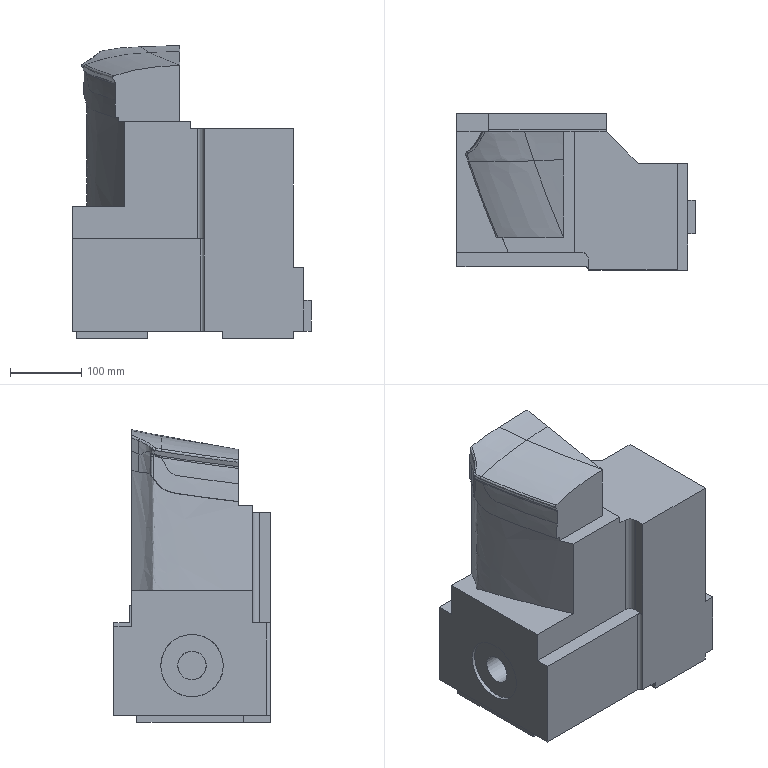Part | NX | features solid 2 | 1 solid | 70 faces | box 335 x 220 x 412.045 mm | volume 17475393 mm3 | plane 41 | spline 25 | cylinder 4 | commonest cylinder face diameters 10 x1 20 x1 40 x1 88 x1